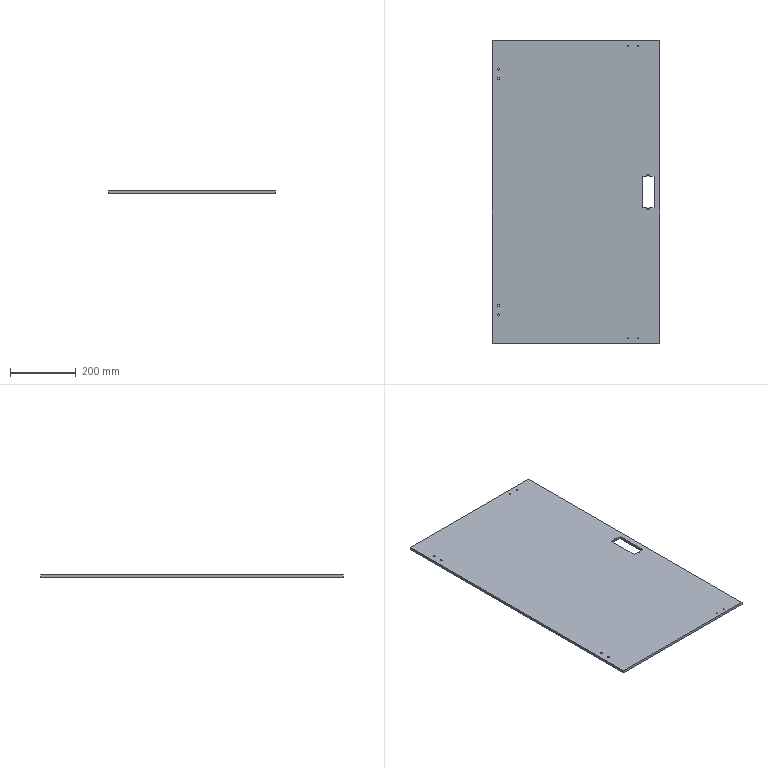Part | STEP file | Left door panel_PN_0007 | 1 solid | 30 faces | box 508.5 x 917 x 8 mm | volume 3700970 mm3 | cylinder 18 | plane 12 | commonest cylinder face diameters 3.3 x8 6.5 x8 8 x2
STEP:
#1=CARTESIAN_POINT('',(-232.,373.5,-4.));
#2=VERTEX_POINT('',#1);
#3=CARTESIAN_POINT('',(-238.5,373.5,-4.));
#4=VERTEX_POINT('',#3);
#5=CARTESIAN_POINT('',(-235.25,373.5,-4.));
#6=DIRECTION('',(0.,0.,-1.));
#7=DIRECTION('',(1.,0.,0.));
#8=AXIS2_PLACEMENT_3D('',#5,#6,#7);
#9=CIRCLE('',#8,3.25);
#10=EDGE_CURVE('',#2,#4,#9,.T.);
#11=ORIENTED_EDGE('',*,*,#10,.T.);
#12=CARTESIAN_POINT('',(-238.5,373.5,4.));
#13=VERTEX_POINT('',#12);
#14=CARTESIAN_POINT('',(-238.5,373.5,-4.));
#15=DIRECTION('',(0.,0.,1.));
#16=VECTOR('',#15,1000.);
#17=LINE('',#14,#16);
#18=EDGE_CURVE('',#4,#13,#17,.T.);
#19=ORIENTED_EDGE('',*,*,#18,.T.);
#20=CARTESIAN_POINT('',(-232.,373.5,4.));
#21=VERTEX_POINT('',#20);
#22=CARTESIAN_POINT('',(-235.25,373.5,4.));
#23=DIRECTION('',(0.,0.,-1.));
#24=DIRECTION('',(1.,0.,0.));
#25=AXIS2_PLACEMENT_3D('',#22,#23,#24);
#26=CIRCLE('',#25,3.25);
#27=EDGE_CURVE('',#21,#13,#26,.T.);
#28=ORIENTED_EDGE('',*,*,#27,.F.);
#29=CARTESIAN_POINT('',(-232.,373.5,-4.));
#30=DIRECTION('',(0.,0.,1.));
#31=VECTOR('',#30,1000.);
#32=LINE('',#29,#31);
#33=EDGE_CURVE('',#2,#21,#32,.T.);
#34=ORIENTED_EDGE('',*,*,#33,.F.);
#35=EDGE_LOOP('',(#11,#19,#28,#34));
#36=FACE_OUTER_BOUND('',#35,.T.);
#37=CARTESIAN_POINT('',(-235.25,373.5,-4.));
#38=DIRECTION('',(0.,0.,1.));
#39=DIRECTION('',(1.,0.,0.));
#40=AXIS2_PLACEMENT_3D('',#37,#38,#39);
#41=CYLINDRICAL_SURFACE('',#40,3.25);
#42=ADVANCED_FACE('',(#36),#41,.F.);
#43=CARTESIAN_POINT('',(-232.,343.5,-4.));
#44=VERTEX_POINT('',#43);
#45=CARTESIAN_POINT('',(-238.5,343.5,-4.));
#46=VERTEX_POINT('',#45);
#47=CARTESIAN_POINT('',(-235.25,343.5,-4.));
#48=DIRECTION('',(0.,0.,-1.));
#49=DIRECTION('',(1.,0.,0.));
#50=AXIS2_PLACEMENT_3D('',#47,#48,#49);
#51=CIRCLE('',#50,3.25);
#52=EDGE_CURVE('',#44,#46,#51,.T.);
#53=ORIENTED_EDGE('',*,*,#52,.T.);
#54=CARTESIAN_POINT('',(-238.5,343.5,4.));
#55=VERTEX_POINT('',#54);
#56=CARTESIAN_POINT('',(-238.5,343.5,-4.));
#57=DIRECTION('',(0.,0.,1.));
#58=VECTOR('',#57,1000.);
#59=LINE('',#56,#58);
#60=EDGE_CURVE('',#46,#55,#59,.T.);
#61=ORIENTED_EDGE('',*,*,#60,.T.);
#62=CARTESIAN_POINT('',(-232.,343.5,4.));
#63=VERTEX_POINT('',#62);
#64=CARTESIAN_POINT('',(-235.25,343.5,4.));
#65=DIRECTION('',(0.,0.,-1.));
#66=DIRECTION('',(1.,0.,0.));
#67=AXIS2_PLACEMENT_3D('',#64,#65,#66);
#68=CIRCLE('',#67,3.25);
#69=EDGE_CURVE('',#63,#55,#68,.T.);
#70=ORIENTED_EDGE('',*,*,#69,.F.);
#71=CARTESIAN_POINT('',(-232.,343.5,-4.));
#72=DIRECTION('',(0.,0.,1.));
#73=VECTOR('',#72,1000.);
#74=LINE('',#71,#73);
#75=EDGE_CURVE('',#44,#63,#74,.T.);
#76=ORIENTED_EDGE('',*,*,#75,.F.);
#77=EDGE_LOOP('',(#53,#61,#70,#76));
#78=FACE_OUTER_BOUND('',#77,.T.);
#79=CARTESIAN_POINT('',(-235.25,343.5,-4.));
#80=DIRECTION('',(0.,0.,1.));
#81=DIRECTION('',(1.,0.,0.));
#82=AXIS2_PLACEMENT_3D('',#79,#80,#81);
#83=CYLINDRICAL_SURFACE('',#82,3.25);
#84=ADVANCED_FACE('',(#78),#83,.F.);
#85=CARTESIAN_POINT('',(-232.,-343.5,-4.));
#86=VERTEX_POINT('',#85);
#87=CARTESIAN_POINT('',(-238.5,-343.5,-4.));
#88=VERTEX_POINT('',#87);
#89=CARTESIAN_POINT('',(-235.25,-343.5,-4.));
#90=DIRECTION('',(0.,0.,-1.));
#91=DIRECTION('',(1.,0.,0.));
#92=AXIS2_PLACEMENT_3D('',#89,#90,#91);
#93=CIRCLE('',#92,3.25);
#94=EDGE_CURVE('',#86,#88,#93,.T.);
#95=ORIENTED_EDGE('',*,*,#94,.T.);
#96=CARTESIAN_POINT('',(-238.5,-343.5,4.));
#97=VERTEX_POINT('',#96);
#98=CARTESIAN_POINT('',(-238.5,-343.5,-4.));
#99=DIRECTION('',(0.,0.,1.));
#100=VECTOR('',#99,1000.);
#101=LINE('',#98,#100);
#102=EDGE_CURVE('',#88,#97,#101,.T.);
#103=ORIENTED_EDGE('',*,*,#102,.T.);
#104=CARTESIAN_POINT('',(-232.,-343.5,4.));
#105=VERTEX_POINT('',#104);
#106=CARTESIAN_POINT('',(-235.25,-343.5,4.));
#107=DIRECTION('',(0.,0.,-1.));
#108=DIRECTION('',(1.,0.,0.));
#109=AXIS2_PLACEMENT_3D('',#106,#107,#108);
#110=CIRCLE('',#109,3.25);
#111=EDGE_CURVE('',#105,#97,#110,.T.);
#112=ORIENTED_EDGE('',*,*,#111,.F.);
#113=CARTESIAN_POINT('',(-232.,-343.5,-4.));
#114=DIRECTION('',(0.,0.,1.));
#115=VECTOR('',#114,1000.);
#116=LINE('',#113,#115);
#117=EDGE_CURVE('',#86,#105,#116,.T.);
#118=ORIENTED_EDGE('',*,*,#117,.F.);
#119=EDGE_LOOP('',(#95,#103,#112,#118));
#120=FACE_OUTER_BOUND('',#119,.T.);
#121=CARTESIAN_POINT('',(-235.25,-343.5,-4.));
#122=DIRECTION('',(0.,0.,1.));
#123=DIRECTION('',(1.,0.,0.));
#124=AXIS2_PLACEMENT_3D('',#121,#122,#123);
#125=CYLINDRICAL_SURFACE('',#124,3.25);
#126=ADVANCED_FACE('',(#120),#125,.F.);
#127=CARTESIAN_POINT('',(-232.,-373.5,-4.));
#128=VERTEX_POINT('',#127);
#129=CARTESIAN_POINT('',(-238.5,-373.5,-4.));
#130=VERTEX_POINT('',#129);
#131=CARTESIAN_POINT('',(-235.25,-373.5,-4.));
#132=DIRECTION('',(0.,0.,-1.));
#133=DIRECTION('',(1.,0.,0.));
#134=AXIS2_PLACEMENT_3D('',#131,#132,#133);
#135=CIRCLE('',#134,3.25);
#136=EDGE_CURVE('',#128,#130,#135,.T.);
#137=ORIENTED_EDGE('',*,*,#136,.T.);
#138=CARTESIAN_POINT('',(-238.5,-373.5,4.));
#139=VERTEX_POINT('',#138);
#140=CARTESIAN_POINT('',(-238.5,-373.5,-4.));
#141=DIRECTION('',(0.,0.,1.));
#142=VECTOR('',#141,1000.);
#143=LINE('',#140,#142);
#144=EDGE_CURVE('',#130,#139,#143,.T.);
#145=ORIENTED_EDGE('',*,*,#144,.T.);
#146=CARTESIAN_POINT('',(-232.,-373.5,4.));
#147=VERTEX_POINT('',#146);
#148=CARTESIAN_POINT('',(-235.25,-373.5,4.));
#149=DIRECTION('',(0.,0.,-1.));
#150=DIRECTION('',(1.,0.,0.));
#151=AXIS2_PLACEMENT_3D('',#148,#149,#150);
#152=CIRCLE('',#151,3.25);
#153=EDGE_CURVE('',#147,#139,#152,.T.);
#154=ORIENTED_EDGE('',*,*,#153,.F.);
#155=CARTESIAN_POINT('',(-232.,-373.5,-4.));
#156=DIRECTION('',(0.,0.,1.));
#157=VECTOR('',#156,1000.);
#158=LINE('',#155,#157);
#159=EDGE_CURVE('',#128,#147,#158,.T.);
#160=ORIENTED_EDGE('',*,*,#159,.F.);
#161=EDGE_LOOP('',(#137,#145,#154,#160));
#162=FACE_OUTER_BOUND('',#161,.T.);
#163=CARTESIAN_POINT('',(-235.25,-373.5,-4.));
#164=DIRECTION('',(0.,0.,1.));
#165=DIRECTION('',(1.,0.,0.));
#166=AXIS2_PLACEMENT_3D('',#163,#164,#165);
#167=CYLINDRICAL_SURFACE('',#166,3.25);
#168=ADVANCED_FACE('',(#162),#167,.F.);
#169=CARTESIAN_POINT('',(160.9,-444.5,4.));
#170=VERTEX_POINT('',#169);
#171=CARTESIAN_POINT('',(157.6,-444.5,4.));
#172=VERTEX_POINT('',#171);
#173=CARTESIAN_POINT('',(159.25,-444.5,4.));
#174=DIRECTION('',(0.,0.,-1.));
#175=DIRECTION('',(-1.,0.,0.));
#176=AXIS2_PLACEMENT_3D('',#173,#174,#175);
#177=CIRCLE('',#176,1.65);
#178=EDGE_CURVE('',#170,#172,#177,.T.);
#179=ORIENTED_EDGE('',*,*,#178,.F.);
#180=CARTESIAN_POINT('',(160.9,-444.5,-4.));
#181=VERTEX_POINT('',#180);
#182=CARTESIAN_POINT('',(160.9,-444.5,-4.));
#183=DIRECTION('',(0.,0.,-1.));
#184=VECTOR('',#183,1000.);
#185=LINE('',#182,#184);
#186=EDGE_CURVE('',#170,#181,#185,.T.);
#187=ORIENTED_EDGE('',*,*,#186,.T.);
#188=CARTESIAN_POINT('',(157.6,-444.5,-4.));
#189=VERTEX_POINT('',#188);
#190=CARTESIAN_POINT('',(159.25,-444.5,-4.));
#191=DIRECTION('',(0.,0.,-1.));
#192=DIRECTION('',(-1.,0.,0.));
#193=AXIS2_PLACEMENT_3D('',#190,#191,#192);
#194=CIRCLE('',#193,1.65);
#195=EDGE_CURVE('',#181,#189,#194,.T.);
#196=ORIENTED_EDGE('',*,*,#195,.T.);
#197=CARTESIAN_POINT('',(157.6,-444.5,-4.));
#198=DIRECTION('',(0.,0.,-1.));
#199=VECTOR('',#198,1000.);
#200=LINE('',#197,#199);
#201=EDGE_CURVE('',#172,#189,#200,.T.);
#202=ORIENTED_EDGE('',*,*,#201,.F.);
#203=EDGE_LOOP('',(#179,#187,#196,#202));
#204=FACE_OUTER_BOUND('',#203,.T.);
#205=CARTESIAN_POINT('',(159.25,-444.5,-4.));
#206=DIRECTION('',(0.,0.,-1.));
#207=DIRECTION('',(-1.,0.,0.));
#208=AXIS2_PLACEMENT_3D('',#205,#206,#207);
#209=CYLINDRICAL_SURFACE('',#208,1.65);
#210=ADVANCED_FACE('',(#204),#209,.F.);
#211=CARTESIAN_POINT('',(190.9,-444.5,4.));
#212=VERTEX_POINT('',#211);
#213=CARTESIAN_POINT('',(187.6,-444.5,4.));
#214=VERTEX_POINT('',#213);
#215=CARTESIAN_POINT('',(189.25,-444.5,4.));
#216=DIRECTION('',(0.,0.,-1.));
#217=DIRECTION('',(-1.,0.,0.));
#218=AXIS2_PLACEMENT_3D('',#215,#216,#217);
#219=CIRCLE('',#218,1.65);
#220=EDGE_CURVE('',#212,#214,#219,.T.);
#221=ORIENTED_EDGE('',*,*,#220,.F.);
#222=CARTESIAN_POINT('',(190.9,-444.5,-4.));
#223=VERTEX_POINT('',#222);
#224=CARTESIAN_POINT('',(190.9,-444.5,-4.));
#225=DIRECTION('',(0.,0.,-1.));
#226=VECTOR('',#225,1000.);
#227=LINE('',#224,#226);
#228=EDGE_CURVE('',#212,#223,#227,.T.);
#229=ORIENTED_EDGE('',*,*,#228,.T.);
#230=CARTESIAN_POINT('',(187.6,-444.5,-4.));
#231=VERTEX_POINT('',#230);
#232=CARTESIAN_POINT('',(189.25,-444.5,-4.));
#233=DIRECTION('',(0.,0.,-1.));
#234=DIRECTION('',(-1.,0.,0.));
#235=AXIS2_PLACEMENT_3D('',#232,#233,#234);
#236=CIRCLE('',#235,1.65);
#237=EDGE_CURVE('',#223,#231,#236,.T.);
#238=ORIENTED_EDGE('',*,*,#237,.T.);
#239=CARTESIAN_POINT('',(187.6,-444.5,-4.));
#240=DIRECTION('',(0.,0.,-1.));
#241=VECTOR('',#240,1000.);
#242=LINE('',#239,#241);
#243=EDGE_CURVE('',#214,#231,#242,.T.);
#244=ORIENTED_EDGE('',*,*,#243,.F.);
#245=EDGE_LOOP('',(#221,#229,#238,#244));
#246=FACE_OUTER_BOUND('',#245,.T.);
#247=CARTESIAN_POINT('',(189.25,-444.5,-4.));
#248=DIRECTION('',(0.,0.,-1.));
#249=DIRECTION('',(-1.,0.,0.));
#250=AXIS2_PLACEMENT_3D('',#247,#248,#249);
#251=CYLINDRICAL_SURFACE('',#250,1.65);
#252=ADVANCED_FACE('',(#246),#251,.F.);
#253=CARTESIAN_POINT('',(160.9,443.5,4.));
#254=VERTEX_POINT('',#253);
#255=CARTESIAN_POINT('',(157.6,443.5,4.));
#256=VERTEX_POINT('',#255);
#257=CARTESIAN_POINT('',(159.25,443.5,4.));
#258=DIRECTION('',(0.,0.,-1.));
#259=DIRECTION('',(-1.,0.,0.));
#260=AXIS2_PLACEMENT_3D('',#257,#258,#259);
#261=CIRCLE('',#260,1.65);
#262=EDGE_CURVE('',#254,#256,#261,.T.);
#263=ORIENTED_EDGE('',*,*,#262,.F.);
#264=CARTESIAN_POINT('',(160.9,443.5,-4.));
#265=VERTEX_POINT('',#264);
#266=CARTESIAN_POINT('',(160.9,443.5,-4.));
#267=DIRECTION('',(0.,0.,-1.));
#268=VECTOR('',#267,1000.);
#269=LINE('',#266,#268);
#270=EDGE_CURVE('',#254,#265,#269,.T.);
#271=ORIENTED_EDGE('',*,*,#270,.T.);
#272=CARTESIAN_POINT('',(157.6,443.5,-4.));
#273=VERTEX_POINT('',#272);
#274=CARTESIAN_POINT('',(159.25,443.5,-4.));
#275=DIRECTION('',(0.,0.,-1.));
#276=DIRECTION('',(-1.,0.,0.));
#277=AXIS2_PLACEMENT_3D('',#274,#275,#276);
#278=CIRCLE('',#277,1.65);
#279=EDGE_CURVE('',#265,#273,#278,.T.);
#280=ORIENTED_EDGE('',*,*,#279,.T.);
#281=CARTESIAN_POINT('',(157.6,443.5,-4.));
#282=DIRECTION('',(0.,0.,-1.));
#283=VECTOR('',#282,1000.);
#284=LINE('',#281,#283);
#285=EDGE_CURVE('',#256,#273,#284,.T.);
#286=ORIENTED_EDGE('',*,*,#285,.F.);
#287=EDGE_LOOP('',(#263,#271,#280,#286));
#288=FACE_OUTER_BOUND('',#287,.T.);
#289=CARTESIAN_POINT('',(159.25,443.5,-4.));
#290=DIRECTION('',(0.,0.,-1.));
#291=DIRECTION('',(-1.,0.,0.));
#292=AXIS2_PLACEMENT_3D('',#289,#290,#291);
#293=CYLINDRICAL_SURFACE('',#292,1.65);
#294=ADVANCED_FACE('',(#288),#293,.F.);
#295=CARTESIAN_POINT('',(190.9,443.5,4.));
#296=VERTEX_POINT('',#295);
#297=CARTESIAN_POINT('',(187.6,443.5,4.));
#298=VERTEX_POINT('',#297);
#299=CARTESIAN_POINT('',(189.25,443.5,4.));
#300=DIRECTION('',(0.,0.,-1.));
#301=DIRECTION('',(-1.,0.,0.));
#302=AXIS2_PLACEMENT_3D('',#299,#300,#301);
#303=CIRCLE('',#302,1.65);
#304=EDGE_CURVE('',#296,#298,#303,.T.);
#305=ORIENTED_EDGE('',*,*,#304,.F.);
#306=CARTESIAN_POINT('',(190.9,443.5,-4.));
#307=VERTEX_POINT('',#306);
#308=CARTESIAN_POINT('',(190.9,443.5,-4.));
#309=DIRECTION('',(0.,0.,-1.));
#310=VECTOR('',#309,1000.);
#311=LINE('',#308,#310);
#312=EDGE_CURVE('',#296,#307,#311,.T.);
#313=ORIENTED_EDGE('',*,*,#312,.T.);
#314=CARTESIAN_POINT('',(187.6,443.5,-4.));
#315=VERTEX_POINT('',#314);
#316=CARTESIAN_POINT('',(189.25,443.5,-4.));
#317=DIRECTION('',(0.,0.,-1.));
#318=DIRECTION('',(-1.,0.,0.));
#319=AXIS2_PLACEMENT_3D('',#316,#317,#318);
#320=CIRCLE('',#319,1.65);
#321=EDGE_CURVE('',#307,#315,#320,.T.);
#322=ORIENTED_EDGE('',*,*,#321,.T.);
#323=CARTESIAN_POINT('',(187.6,443.5,-4.));
#324=DIRECTION('',(0.,0.,-1.));
#325=VECTOR('',#324,1000.);
#326=LINE('',#323,#325);
#327=EDGE_CURVE('',#298,#315,#326,.T.);
#328=ORIENTED_EDGE('',*,*,#327,.F.);
#329=EDGE_LOOP('',(#305,#313,#322,#328));
#330=FACE_OUTER_BOUND('',#329,.T.);
#331=CARTESIAN_POINT('',(189.25,443.5,-4.));
#332=DIRECTION('',(0.,0.,-1.));
#333=DIRECTION('',(-1.,0.,0.));
#334=AXIS2_PLACEMENT_3D('',#331,#332,#333);
#335=CYLINDRICAL_SURFACE('',#334,1.65);
#336=ADVANCED_FACE('',(#330),#335,.F.);
#337=CARTESIAN_POINT('',(215.25,48.,-4.));
#338=VERTEX_POINT('',#337);
#339=CARTESIAN_POINT('',(223.25,48.,-4.));
#340=VERTEX_POINT('',#339);
#341=CARTESIAN_POINT('',(219.25,48.,-4.));
#342=DIRECTION('',(0.,0.,-1.));
#343=DIRECTION('',(1.,0.,0.));
#344=AXIS2_PLACEMENT_3D('',#341,#342,#343);
#345=CIRCLE('',#344,4.);
#346=EDGE_CURVE('',#338,#340,#345,.T.);
#347=ORIENTED_EDGE('',*,*,#346,.F.);
#348=CARTESIAN_POINT('',(201.25,48.,-4.));
#349=VERTEX_POINT('',#348);
#350=CARTESIAN_POINT('',(0.,48.,-4.));
#351=DIRECTION('',(1.,0.,0.));
#352=VECTOR('',#351,1000.);
#353=LINE('',#350,#352);
#354=EDGE_CURVE('',#349,#338,#353,.T.);
#355=ORIENTED_EDGE('',*,*,#354,.F.);
#356=CARTESIAN_POINT('',(201.25,-48.,-4.));
#357=VERTEX_POINT('',#356);
#358=CARTESIAN_POINT('',(201.25,0.,-4.));
#359=DIRECTION('',(0.,1.,0.));
#360=VECTOR('',#359,1000.);
#361=LINE('',#358,#360);
#362=EDGE_CURVE('',#357,#349,#361,.T.);
#363=ORIENTED_EDGE('',*,*,#362,.F.);
#364=CARTESIAN_POINT('',(215.25,-48.,-4.));
#365=VERTEX_POINT('',#364);
#366=CARTESIAN_POINT('',(0.,-48.,-4.));
#367=DIRECTION('',(-1.,0.,0.));
#368=VECTOR('',#367,1000.);
#369=LINE('',#366,#368);
#370=EDGE_CURVE('',#365,#357,#369,.T.);
#371=ORIENTED_EDGE('',*,*,#370,.F.);
#372=CARTESIAN_POINT('',(223.25,-48.,-4.));
#373=VERTEX_POINT('',#372);
#374=CARTESIAN_POINT('',(219.25,-48.,-4.));
#375=DIRECTION('',(0.,0.,-1.));
#376=DIRECTION('',(1.,0.,0.));
#377=AXIS2_PLACEMENT_3D('',#374,#375,#376);
#378=CIRCLE('',#377,4.);
#379=EDGE_CURVE('',#373,#365,#378,.T.);
#380=ORIENTED_EDGE('',*,*,#379,.F.);
#381=CARTESIAN_POINT('',(237.25,-48.,-4.));
#382=VERTEX_POINT('',#381);
#383=CARTESIAN_POINT('',(0.,-48.,-4.));
#384=DIRECTION('',(-1.,0.,0.));
#385=VECTOR('',#384,1000.);
#386=LINE('',#383,#385);
#387=EDGE_CURVE('',#382,#373,#386,.T.);
#388=ORIENTED_EDGE('',*,*,#387,.F.);
#389=CARTESIAN_POINT('',(237.25,48.,-4.));
#390=VERTEX_POINT('',#389);
#391=CARTESIAN_POINT('',(237.25,0.,-4.));
#392=DIRECTION('',(0.,-1.,0.));
#393=VECTOR('',#392,1000.);
#394=LINE('',#391,#393);
#395=EDGE_CURVE('',#390,#382,#394,.T.);
#396=ORIENTED_EDGE('',*,*,#395,.F.);
#397=CARTESIAN_POINT('',(0.,48.,-4.));
#398=DIRECTION('',(1.,0.,0.));
#399=VECTOR('',#398,1000.);
#400=LINE('',#397,#399);
#401=EDGE_CURVE('',#340,#390,#400,.T.);
#402=ORIENTED_EDGE('',*,*,#401,.F.);
#403=EDGE_LOOP('',(#347,#355,#363,#371,#380,#388,#396,#402));
#404=FACE_BOUND('',#403,.T.);
#405=CARTESIAN_POINT('',(-254.25,-458.5,-4.));
#406=VERTEX_POINT('',#405);
#407=CARTESIAN_POINT('',(254.25,-458.5,-4.));
#408=VERTEX_POINT('',#407);
#409=CARTESIAN_POINT('',(0.,-458.5,-4.));
#410=DIRECTION('',(1.,0.,0.));
#411=VECTOR('',#410,1000.);
#412=LINE('',#409,#411);
#413=EDGE_CURVE('',#406,#408,#412,.T.);
#414=ORIENTED_EDGE('',*,*,#413,.F.);
#415=CARTESIAN_POINT('',(-254.25,458.5,-4.));
#416=VERTEX_POINT('',#415);
#417=CARTESIAN_POINT('',(-254.25,0.,-4.));
#418=DIRECTION('',(0.,-1.,0.));
#419=VECTOR('',#418,1000.);
#420=LINE('',#417,#419);
#421=EDGE_CURVE('',#416,#406,#420,.T.);
#422=ORIENTED_EDGE('',*,*,#421,.F.);
#423=CARTESIAN_POINT('',(254.25,458.5,-4.));
#424=VERTEX_POINT('',#423);
#425=CARTESIAN_POINT('',(0.,458.5,-4.));
#426=DIRECTION('',(-1.,0.,0.));
#427=VECTOR('',#426,1000.);
#428=LINE('',#425,#427);
#429=EDGE_CURVE('',#424,#416,#428,.T.);
#430=ORIENTED_EDGE('',*,*,#429,.F.);
#431=CARTESIAN_POINT('',(254.25,0.,-4.));
#432=DIRECTION('',(0.,1.,0.));
#433=VECTOR('',#432,1000.);
#434=LINE('',#431,#433);
#435=EDGE_CURVE('',#408,#424,#434,.T.);
#436=ORIENTED_EDGE('',*,*,#435,.F.);
#437=EDGE_LOOP('',(#414,#422,#430,#436));
#438=FACE_OUTER_BOUND('',#437,.T.);
#439=ORIENTED_EDGE('',*,*,#10,.F.);
#440=CARTESIAN_POINT('',(-235.25,373.5,-4.));
#441=DIRECTION('',(0.,0.,-1.));
#442=DIRECTION('',(1.,0.,0.));
#443=AXIS2_PLACEMENT_3D('',#440,#441,#442);
#444=CIRCLE('',#443,3.25);
#445=EDGE_CURVE('',#4,#2,#444,.T.);
#446=ORIENTED_EDGE('',*,*,#445,.F.);
#447=EDGE_LOOP('',(#439,#446));
#448=FACE_BOUND('',#447,.T.);
#449=ORIENTED_EDGE('',*,*,#52,.F.);
#450=CARTESIAN_POINT('',(-235.25,343.5,-4.));
#451=DIRECTION('',(0.,0.,-1.));
#452=DIRECTION('',(1.,0.,0.));
#453=AXIS2_PLACEMENT_3D('',#450,#451,#452);
#454=CIRCLE('',#453,3.25);
#455=EDGE_CURVE('',#46,#44,#454,.T.);
#456=ORIENTED_EDGE('',*,*,#455,.F.);
#457=EDGE_LOOP('',(#449,#456));
#458=FACE_BOUND('',#457,.T.);
#459=ORIENTED_EDGE('',*,*,#94,.F.);
#460=CARTESIAN_POINT('',(-235.25,-343.5,-4.));
#461=DIRECTION('',(0.,0.,-1.));
#462=DIRECTION('',(1.,0.,0.));
#463=AXIS2_PLACEMENT_3D('',#460,#461,#462);
#464=CIRCLE('',#463,3.25);
#465=EDGE_CURVE('',#88,#86,#464,.T.);
#466=ORIENTED_EDGE('',*,*,#465,.F.);
#467=EDGE_LOOP('',(#459,#466));
#468=FACE_BOUND('',#467,.T.);
#469=ORIENTED_EDGE('',*,*,#136,.F.);
#470=CARTESIAN_POINT('',(-235.25,-373.5,-4.));
#471=DIRECTION('',(0.,0.,-1.));
#472=DIRECTION('',(1.,0.,0.));
#473=AXIS2_PLACEMENT_3D('',#470,#471,#472);
#474=CIRCLE('',#473,3.25);
#475=EDGE_CURVE('',#130,#128,#474,.T.);
#476=ORIENTED_EDGE('',*,*,#475,.F.);
#477=EDGE_LOOP('',(#469,#476));
#478=FACE_BOUND('',#477,.T.);
#479=CARTESIAN_POINT('',(159.25,-444.5,-4.));
#480=DIRECTION('',(0.,0.,-1.));
#481=DIRECTION('',(-1.,0.,0.));
#482=AXIS2_PLACEMENT_3D('',#479,#480,#481);
#483=CIRCLE('',#482,1.65);
#484=EDGE_CURVE('',#189,#181,#483,.T.);
#485=ORIENTED_EDGE('',*,*,#484,.F.);
#486=ORIENTED_EDGE('',*,*,#195,.F.);
#487=EDGE_LOOP('',(#485,#486));
#488=FACE_BOUND('',#487,.T.);
#489=CARTESIAN_POINT('',(189.25,-444.5,-4.));
#490=DIRECTION('',(0.,0.,-1.));
#491=DIRECTION('',(-1.,0.,0.));
#492=AXIS2_PLACEMENT_3D('',#489,#490,#491);
#493=CIRCLE('',#492,1.65);
#494=EDGE_CURVE('',#231,#223,#493,.T.);
#495=ORIENTED_EDGE('',*,*,#494,.F.);
#496=ORIENTED_EDGE('',*,*,#237,.F.);
#497=EDGE_LOOP('',(#495,#496));
#498=FACE_BOUND('',#497,.T.);
#499=CARTESIAN_POINT('',(159.25,443.5,-4.));
#500=DIRECTION('',(0.,0.,-1.));
#501=DIRECTION('',(-1.,0.,0.));
#502=AXIS2_PLACEMENT_3D('',#499,#500,#501);
#503=CIRCLE('',#502,1.65);
#504=EDGE_CURVE('',#273,#265,#503,.T.);
#505=ORIENTED_EDGE('',*,*,#504,.F.);
#506=ORIENTED_EDGE('',*,*,#279,.F.);
#507=EDGE_LOOP('',(#505,#506));
#508=FACE_BOUND('',#507,.T.);
#509=CARTESIAN_POINT('',(189.25,443.5,-4.));
#510=DIRECTION('',(0.,0.,-1.));
#511=DIRECTION('',(-1.,0.,0.));
#512=AXIS2_PLACEMENT_3D('',#509,#510,#511);
#513=CIRCLE('',#512,1.65);
#514=EDGE_CURVE('',#315,#307,#513,.T.);
#515=ORIENTED_EDGE('',*,*,#514,.F.);
#516=ORIENTED_EDGE('',*,*,#321,.F.);
#517=EDGE_LOOP('',(#515,#516));
#518=FACE_BOUND('',#517,.T.);
#519=CARTESIAN_POINT('',(0.,0.,-4.));
#520=DIRECTION('',(0.,0.,1.));
#521=DIRECTION('',(1.,0.,0.));
#522=AXIS2_PLACEMENT_3D('',#519,#520,#521);
#523=PLANE('',#522);
#524=ADVANCED_FACE('',(#404,#438,#448,#458,#468,#478,#488,#498,#508,#518),#523,.F.);
#525=ORIENTED_EDGE('',*,*,#401,.T.);
#526=CARTESIAN_POINT('',(237.25,48.,4.));
#527=VERTEX_POINT('',#526);
#528=CARTESIAN_POINT('',(237.25,48.,-4.));
#529=DIRECTION('',(0.,0.,1.));
#530=VECTOR('',#529,1000.);
#531=LINE('',#528,#530);
#532=EDGE_CURVE('',#390,#527,#531,.T.);
#533=ORIENTED_EDGE('',*,*,#532,.T.);
#534=CARTESIAN_POINT('',(223.25,48.,4.));
#535=VERTEX_POINT('',#534);
#536=CARTESIAN_POINT('',(0.,48.,4.));
#537=DIRECTION('',(-1.,0.,0.));
#538=VECTOR('',#537,1000.);
#539=LINE('',#536,#538);
#540=EDGE_CURVE('',#527,#535,#539,.T.);
#541=ORIENTED_EDGE('',*,*,#540,.T.);
#542=CARTESIAN_POINT('',(223.25,48.,-4.));
#543=DIRECTION('',(0.,0.,-1.));
#544=VECTOR('',#543,1000.);
#545=LINE('',#542,#544);
#546=EDGE_CURVE('',#535,#340,#545,.T.);
#547=ORIENTED_EDGE('',*,*,#546,.T.);
#548=EDGE_LOOP('',(#525,#533,#541,#547));
#549=FACE_OUTER_BOUND('',#548,.T.);
#550=CARTESIAN_POINT('',(0.,48.,-4.));
#551=DIRECTION('',(0.,-1.,0.));
#552=DIRECTION('',(1.,0.,0.));
#553=AXIS2_PLACEMENT_3D('',#550,#551,#552);
#554=PLANE('',#553);
#555=ADVANCED_FACE('',(#549),#554,.T.);
#556=CARTESIAN_POINT('',(215.25,48.,4.));
#557=VERTEX_POINT('',#556);
#558=CARTESIAN_POINT('',(215.25,48.,-4.));
#559=DIRECTION('',(0.,0.,1.));
#560=VECTOR('',#559,1000.);
#561=LINE('',#558,#560);
#562=EDGE_CURVE('',#338,#557,#561,.T.);
#563=ORIENTED_EDGE('',*,*,#562,.F.);
#564=ORIENTED_EDGE('',*,*,#346,.T.);
#565=ORIENTED_EDGE('',*,*,#546,.F.);
#566=CARTESIAN_POINT('',(219.25,48.,4.));
#567=DIRECTION('',(0.,0.,-1.));
#568=DIRECTION('',(1.,0.,0.));
#569=AXIS2_PLACEMENT_3D('',#566,#567,#568);
#570=CIRCLE('',#569,4.);
#571=EDGE_CURVE('',#557,#535,#570,.T.);
#572=ORIENTED_EDGE('',*,*,#571,.F.);
#573=EDGE_LOOP('',(#563,#564,#565,#572));
#574=FACE_OUTER_BOUND('',#573,.T.);
#575=CARTESIAN_POINT('',(219.25,48.,-4.));
#576=DIRECTION('',(0.,0.,1.));
#577=DIRECTION('',(1.,0.,0.));
#578=AXIS2_PLACEMENT_3D('',#575,#576,#577);
#579=CYLINDRICAL_SURFACE('',#578,4.);
#580=ADVANCED_FACE('',(#574),#579,.F.);
#581=ORIENTED_EDGE('',*,*,#354,.T.);
#582=ORIENTED_EDGE('',*,*,#562,.T.);
#583=CARTESIAN_POINT('',(201.25,48.,4.));
#584=VERTEX_POINT('',#583);
#585=CARTESIAN_POINT('',(0.,48.,4.));
#586=DIRECTION('',(-1.,0.,0.));
#587=VECTOR('',#586,1000.);
#588=LINE('',#585,#587);
#589=EDGE_CURVE('',#557,#584,#588,.T.);
#590=ORIENTED_EDGE('',*,*,#589,.T.);
#591=CARTESIAN_POINT('',(201.25,48.,-4.));
#592=DIRECTION('',(0.,0.,-1.));
#593=VECTOR('',#592,1000.);
#594=LINE('',#591,#593);
#595=EDGE_CURVE('',#584,#349,#594,.T.);
#596=ORIENTED_EDGE('',*,*,#595,.T.);
#597=EDGE_LOOP('',(#581,#582,#590,#596));
#598=FACE_OUTER_BOUND('',#597,.T.);
#599=CARTESIAN_POINT('',(0.,48.,-4.));
#600=DIRECTION('',(0.,-1.,0.));
#601=DIRECTION('',(0.,0.,-1.));
#602=AXIS2_PLACEMENT_3D('',#599,#600,#601);
#603=PLANE('',#602);
#604=ADVANCED_FACE('',(#598),#603,.T.);
#605=CARTESIAN_POINT('',(201.25,-48.,4.));
#606=VERTEX_POINT('',#605);
#607=CARTESIAN_POINT('',(201.25,-48.,-4.));
#608=DIRECTION('',(0.,0.,1.));
#609=VECTOR('',#608,1000.);
#610=LINE('',#607,#609);
#611=EDGE_CURVE('',#357,#606,#610,.T.);
#612=ORIENTED_EDGE('',*,*,#611,.F.);
#613=ORIENTED_EDGE('',*,*,#362,.T.);
#614=ORIENTED_EDGE('',*,*,#595,.F.);
#615=CARTESIAN_POINT('',(201.25,0.,4.));
#616=DIRECTION('',(0.,1.,0.));
#617=VECTOR('',#616,1000.);
#618=LINE('',#615,#617);
#619=EDGE_CURVE('',#606,#584,#618,.T.);
#620=ORIENTED_EDGE('',*,*,#619,.F.);
#621=EDGE_LOOP('',(#612,#613,#614,#620));
#622=FACE_OUTER_BOUND('',#621,.T.);
#623=CARTESIAN_POINT('',(201.25,0.,-4.));
#624=DIRECTION('',(-1.,0.,0.));
#625=DIRECTION('',(0.,-1.,0.));
#626=AXIS2_PLACEMENT_3D('',#623,#624,#625);
#627=PLANE('',#626);
#628=ADVANCED_FACE('',(#622),#627,.F.);
#629=CARTESIAN_POINT('',(215.25,-48.,4.));
#630=VERTEX_POINT('',#629);
#631=CARTESIAN_POINT('',(215.25,-48.,-4.));
#632=DIRECTION('',(0.,0.,1.));
#633=VECTOR('',#632,1000.);
#634=LINE('',#631,#633);
#635=EDGE_CURVE('',#365,#630,#634,.T.);
#636=ORIENTED_EDGE('',*,*,#635,.F.);
#637=ORIENTED_EDGE('',*,*,#370,.T.);
#638=ORIENTED_EDGE('',*,*,#611,.T.);
#639=CARTESIAN_POINT('',(0.,-48.,4.));
#640=DIRECTION('',(-1.,0.,0.));
#641=VECTOR('',#640,1000.);
#642=LINE('',#639,#641);
#643=EDGE_CURVE('',#630,#606,#642,.T.);
#644=ORIENTED_EDGE('',*,*,#643,.F.);
#645=EDGE_LOOP('',(#636,#637,#638,#644));
#646=FACE_OUTER_BOUND('',#645,.T.);
#647=CARTESIAN_POINT('',(0.,-48.,-4.));
#648=DIRECTION('',(0.,-1.,0.));
#649=DIRECTION('',(0.,0.,-1.));
#650=AXIS2_PLACEMENT_3D('',#647,#648,#649);
#651=PLANE('',#650);
#652=ADVANCED_FACE('',(#646),#651,.F.);
#653=CARTESIAN_POINT('',(223.25,-48.,4.));
#654=VERTEX_POINT('',#653);
#655=CARTESIAN_POINT('',(223.25,-48.,-4.));
#656=DIRECTION('',(0.,0.,1.));
#657=VECTOR('',#656,1000.);
#658=LINE('',#655,#657);
#659=EDGE_CURVE('',#373,#654,#658,.T.);
#660=ORIENTED_EDGE('',*,*,#659,.F.);
#661=ORIENTED_EDGE('',*,*,#379,.T.);
#662=ORIENTED_EDGE('',*,*,#635,.T.);
#663=CARTESIAN_POINT('',(219.25,-48.,4.));
#664=DIRECTION('',(0.,0.,-1.));
#665=DIRECTION('',(1.,0.,0.));
#666=AXIS2_PLACEMENT_3D('',#663,#664,#665);
#667=CIRCLE('',#666,4.);
#668=EDGE_CURVE('',#654,#630,#667,.T.);
#669=ORIENTED_EDGE('',*,*,#668,.F.);
#670=EDGE_LOOP('',(#660,#661,#662,#669));
#671=FACE_OUTER_BOUND('',#670,.T.);
#672=CARTESIAN_POINT('',(219.25,-48.,-4.));
#673=DIRECTION('',(0.,0.,1.));
#674=DIRECTION('',(1.,0.,0.));
#675=AXIS2_PLACEMENT_3D('',#672,#673,#674);
#676=CYLINDRICAL_SURFACE('',#675,4.);
#677=ADVANCED_FACE('',(#671),#676,.F.);
#678=CARTESIAN_POINT('',(237.25,-48.,4.));
#679=VERTEX_POINT('',#678);
#680=CARTESIAN_POINT('',(237.25,-48.,-4.));
#681=DIRECTION('',(0.,0.,1.));
#682=VECTOR('',#681,1000.);
#683=LINE('',#680,#682);
#684=EDGE_CURVE('',#382,#679,#683,.T.);
#685=ORIENTED_EDGE('',*,*,#684,.F.);
#686=ORIENTED_EDGE('',*,*,#387,.T.);
#687=ORIENTED_EDGE('',*,*,#659,.T.);
#688=CARTESIAN_POINT('',(0.,-48.,4.));
#689=DIRECTION('',(-1.,0.,0.));
#690=VECTOR('',#689,1000.);
#691=LINE('',#688,#690);
#692=EDGE_CURVE('',#679,#654,#691,.T.);
#693=ORIENTED_EDGE('',*,*,#692,.F.);
#694=EDGE_LOOP('',(#685,#686,#687,#693));
#695=FACE_OUTER_BOUND('',#694,.T.);
#696=CARTESIAN_POINT('',(0.,-48.,-4.));
#697=DIRECTION('',(0.,-1.,0.));
#698=DIRECTION('',(0.,0.,-1.));
#699=AXIS2_PLACEMENT_3D('',#696,#697,#698);
#700=PLANE('',#699);
#701=ADVANCED_FACE('',(#695),#700,.F.);
#702=ORIENTED_EDGE('',*,*,#395,.T.);
#703=ORIENTED_EDGE('',*,*,#684,.T.);
#704=CARTESIAN_POINT('',(237.25,0.,4.));
#705=DIRECTION('',(0.,1.,0.));
#706=VECTOR('',#705,1000.);
#707=LINE('',#704,#706);
#708=EDGE_CURVE('',#679,#527,#707,.T.);
#709=ORIENTED_EDGE('',*,*,#708,.T.);
#710=ORIENTED_EDGE('',*,*,#532,.F.);
#711=EDGE_LOOP('',(#702,#703,#709,#710));
#712=FACE_OUTER_BOUND('',#711,.T.);
#713=CARTESIAN_POINT('',(237.25,0.,-4.));
#714=DIRECTION('',(-1.,0.,0.));
#715=DIRECTION('',(0.,-1.,0.));
#716=AXIS2_PLACEMENT_3D('',#713,#714,#715);
#717=PLANE('',#716);
#718=ADVANCED_FACE('',(#712),#717,.T.);
#719=CARTESIAN_POINT('',(254.25,458.5,4.));
#720=VERTEX_POINT('',#719);
#721=CARTESIAN_POINT('',(254.25,458.5,4.));
#722=DIRECTION('',(0.,0.,-1.));
#723=VECTOR('',#722,1000.);
#724=LINE('',#721,#723);
#725=EDGE_CURVE('',#720,#424,#724,.T.);
#726=ORIENTED_EDGE('',*,*,#725,.F.);
#727=CARTESIAN_POINT('',(254.25,-458.5,4.));
#728=VERTEX_POINT('',#727);
#729=CARTESIAN_POINT('',(254.25,458.5,4.));
#730=DIRECTION('',(0.,1.,0.));
#731=VECTOR('',#730,1000.);
#732=LINE('',#729,#731);
#733=EDGE_CURVE('',#728,#720,#732,.T.);
#734=ORIENTED_EDGE('',*,*,#733,.F.);
#735=CARTESIAN_POINT('',(254.25,-458.5,4.));
#736=DIRECTION('',(0.,0.,1.));
#737=VECTOR('',#736,1000.);
#738=LINE('',#735,#737);
#739=EDGE_CURVE('',#408,#728,#738,.T.);
#740=ORIENTED_EDGE('',*,*,#739,.F.);
#741=ORIENTED_EDGE('',*,*,#435,.T.);
#742=EDGE_LOOP('',(#726,#734,#740,#741));
#743=FACE_OUTER_BOUND('',#742,.T.);
#744=CARTESIAN_POINT('',(254.25,458.5,4.));
#745=DIRECTION('',(-1.,0.,0.));
#746=DIRECTION('',(0.,-1.,0.));
#747=AXIS2_PLACEMENT_3D('',#744,#745,#746);
#748=PLANE('',#747);
#749=ADVANCED_FACE('',(#743),#748,.F.);
#750=ORIENTED_EDGE('',*,*,#739,.T.);
#751=CARTESIAN_POINT('',(-254.25,-458.5,4.));
#752=VERTEX_POINT('',#751);
#753=CARTESIAN_POINT('',(-254.25,-458.5,4.));
#754=DIRECTION('',(1.,0.,0.));
#755=VECTOR('',#754,1000.);
#756=LINE('',#753,#755);
#757=EDGE_CURVE('',#752,#728,#756,.T.);
#758=ORIENTED_EDGE('',*,*,#757,.F.);
#759=CARTESIAN_POINT('',(-254.25,-458.5,4.));
#760=DIRECTION('',(0.,0.,1.));
#761=VECTOR('',#760,1000.);
#762=LINE('',#759,#761);
#763=EDGE_CURVE('',#406,#752,#762,.T.);
#764=ORIENTED_EDGE('',*,*,#763,.F.);
#765=ORIENTED_EDGE('',*,*,#413,.T.);
#766=EDGE_LOOP('',(#750,#758,#764,#765));
#767=FACE_OUTER_BOUND('',#766,.T.);
#768=CARTESIAN_POINT('',(-254.25,-458.5,4.));
#769=DIRECTION('',(0.,1.,0.));
#770=DIRECTION('',(0.,0.,1.));
#771=AXIS2_PLACEMENT_3D('',#768,#769,#770);
#772=PLANE('',#771);
#773=ADVANCED_FACE('',(#767),#772,.F.);
#774=ORIENTED_EDGE('',*,*,#763,.T.);
#775=CARTESIAN_POINT('',(-254.25,458.5,4.));
#776=VERTEX_POINT('',#775);
#777=CARTESIAN_POINT('',(-254.25,458.5,4.));
#778=DIRECTION('',(0.,-1.,0.));
#779=VECTOR('',#778,1000.);
#780=LINE('',#777,#779);
#781=EDGE_CURVE('',#776,#752,#780,.T.);
#782=ORIENTED_EDGE('',*,*,#781,.F.);
#783=CARTESIAN_POINT('',(-254.25,458.5,4.));
#784=DIRECTION('',(0.,0.,1.));
#785=VECTOR('',#784,1000.);
#786=LINE('',#783,#785);
#787=EDGE_CURVE('',#416,#776,#786,.T.);
#788=ORIENTED_EDGE('',*,*,#787,.F.);
#789=ORIENTED_EDGE('',*,*,#421,.T.);
#790=EDGE_LOOP('',(#774,#782,#788,#789));
#791=FACE_OUTER_BOUND('',#790,.T.);
#792=CARTESIAN_POINT('',(-254.25,458.5,4.));
#793=DIRECTION('',(1.,0.,0.));
#794=DIRECTION('',(0.,1.,0.));
#795=AXIS2_PLACEMENT_3D('',#792,#793,#794);
#796=PLANE('',#795);
#797=ADVANCED_FACE('',(#791),#796,.F.);
#798=ORIENTED_EDGE('',*,*,#787,.T.);
#799=CARTESIAN_POINT('',(-254.25,458.5,4.));
#800=DIRECTION('',(-1.,0.,0.));
#801=VECTOR('',#800,1000.);
#802=LINE('',#799,#801);
#803=EDGE_CURVE('',#720,#776,#802,.T.);
#804=ORIENTED_EDGE('',*,*,#803,.F.);
#805=ORIENTED_EDGE('',*,*,#725,.T.);
#806=ORIENTED_EDGE('',*,*,#429,.T.);
#807=EDGE_LOOP('',(#798,#804,#805,#806));
#808=FACE_OUTER_BOUND('',#807,.T.);
#809=CARTESIAN_POINT('',(-254.25,458.5,4.));
#810=DIRECTION('',(0.,-1.,0.));
#811=DIRECTION('',(0.,0.,-1.));
#812=AXIS2_PLACEMENT_3D('',#809,#810,#811);
#813=PLANE('',#812);
#814=ADVANCED_FACE('',(#808),#813,.F.);
#815=ORIENTED_EDGE('',*,*,#18,.F.);
#816=ORIENTED_EDGE('',*,*,#445,.T.);
#817=ORIENTED_EDGE('',*,*,#33,.T.);
#818=CARTESIAN_POINT('',(-235.25,373.5,4.));
#819=DIRECTION('',(0.,0.,-1.));
#820=DIRECTION('',(1.,0.,0.));
#821=AXIS2_PLACEMENT_3D('',#818,#819,#820);
#822=CIRCLE('',#821,3.25);
#823=EDGE_CURVE('',#13,#21,#822,.T.);
#824=ORIENTED_EDGE('',*,*,#823,.F.);
#825=EDGE_LOOP('',(#815,#816,#817,#824));
#826=FACE_OUTER_BOUND('',#825,.T.);
#827=CARTESIAN_POINT('',(-235.25,373.5,-4.));
#828=DIRECTION('',(0.,0.,1.));
#829=DIRECTION('',(1.,0.,0.));
#830=AXIS2_PLACEMENT_3D('',#827,#828,#829);
#831=CYLINDRICAL_SURFACE('',#830,3.25);
#832=ADVANCED_FACE('',(#826),#831,.F.);
#833=ORIENTED_EDGE('',*,*,#60,.F.);
#834=ORIENTED_EDGE('',*,*,#455,.T.);
#835=ORIENTED_EDGE('',*,*,#75,.T.);
#836=CARTESIAN_POINT('',(-235.25,343.5,4.));
#837=DIRECTION('',(0.,0.,-1.));
#838=DIRECTION('',(1.,0.,0.));
#839=AXIS2_PLACEMENT_3D('',#836,#837,#838);
#840=CIRCLE('',#839,3.25);
#841=EDGE_CURVE('',#55,#63,#840,.T.);
#842=ORIENTED_EDGE('',*,*,#841,.F.);
#843=EDGE_LOOP('',(#833,#834,#835,#842));
#844=FACE_OUTER_BOUND('',#843,.T.);
#845=CARTESIAN_POINT('',(-235.25,343.5,-4.));
#846=DIRECTION('',(0.,0.,1.));
#847=DIRECTION('',(1.,0.,0.));
#848=AXIS2_PLACEMENT_3D('',#845,#846,#847);
#849=CYLINDRICAL_SURFACE('',#848,3.25);
#850=ADVANCED_FACE('',(#844),#849,.F.);
#851=ORIENTED_EDGE('',*,*,#102,.F.);
#852=ORIENTED_EDGE('',*,*,#465,.T.);
#853=ORIENTED_EDGE('',*,*,#117,.T.);
#854=CARTESIAN_POINT('',(-235.25,-343.5,4.));
#855=DIRECTION('',(0.,0.,-1.));
#856=DIRECTION('',(1.,0.,0.));
#857=AXIS2_PLACEMENT_3D('',#854,#855,#856);
#858=CIRCLE('',#857,3.25);
#859=EDGE_CURVE('',#97,#105,#858,.T.);
#860=ORIENTED_EDGE('',*,*,#859,.F.);
#861=EDGE_LOOP('',(#851,#852,#853,#860));
#862=FACE_OUTER_BOUND('',#861,.T.);
#863=CARTESIAN_POINT('',(-235.25,-343.5,-4.));
#864=DIRECTION('',(0.,0.,1.));
#865=DIRECTION('',(1.,0.,0.));
#866=AXIS2_PLACEMENT_3D('',#863,#864,#865);
#867=CYLINDRICAL_SURFACE('',#866,3.25);
#868=ADVANCED_FACE('',(#862),#867,.F.);
#869=ORIENTED_EDGE('',*,*,#144,.F.);
#870=ORIENTED_EDGE('',*,*,#475,.T.);
#871=ORIENTED_EDGE('',*,*,#159,.T.);
#872=CARTESIAN_POINT('',(-235.25,-373.5,4.));
#873=DIRECTION('',(0.,0.,-1.));
#874=DIRECTION('',(1.,0.,0.));
#875=AXIS2_PLACEMENT_3D('',#872,#873,#874);
#876=CIRCLE('',#875,3.25);
#877=EDGE_CURVE('',#139,#147,#876,.T.);
#878=ORIENTED_EDGE('',*,*,#877,.F.);
#879=EDGE_LOOP('',(#869,#870,#871,#878));
#880=FACE_OUTER_BOUND('',#879,.T.);
#881=CARTESIAN_POINT('',(-235.25,-373.5,-4.));
#882=DIRECTION('',(0.,0.,1.));
#883=DIRECTION('',(1.,0.,0.));
#884=AXIS2_PLACEMENT_3D('',#881,#882,#883);
#885=CYLINDRICAL_SURFACE('',#884,3.25);
#886=ADVANCED_FACE('',(#880),#885,.F.);
#887=ORIENTED_EDGE('',*,*,#186,.F.);
#888=CARTESIAN_POINT('',(159.25,-444.5,4.));
#889=DIRECTION('',(0.,0.,-1.));
#890=DIRECTION('',(-1.,0.,0.));
#891=AXIS2_PLACEMENT_3D('',#888,#889,#890);
#892=CIRCLE('',#891,1.65);
#893=EDGE_CURVE('',#172,#170,#892,.T.);
#894=ORIENTED_EDGE('',*,*,#893,.F.);
#895=ORIENTED_EDGE('',*,*,#201,.T.);
#896=ORIENTED_EDGE('',*,*,#484,.T.);
#897=EDGE_LOOP('',(#887,#894,#895,#896));
#898=FACE_OUTER_BOUND('',#897,.T.);
#899=CARTESIAN_POINT('',(159.25,-444.5,-4.));
#900=DIRECTION('',(0.,0.,-1.));
#901=DIRECTION('',(-1.,0.,0.));
#902=AXIS2_PLACEMENT_3D('',#899,#900,#901);
#903=CYLINDRICAL_SURFACE('',#902,1.65);
#904=ADVANCED_FACE('',(#898),#903,.F.);
#905=ORIENTED_EDGE('',*,*,#228,.F.);
#906=CARTESIAN_POINT('',(189.25,-444.5,4.));
#907=DIRECTION('',(0.,0.,-1.));
#908=DIRECTION('',(-1.,0.,0.));
#909=AXIS2_PLACEMENT_3D('',#906,#907,#908);
#910=CIRCLE('',#909,1.65);
#911=EDGE_CURVE('',#214,#212,#910,.T.);
#912=ORIENTED_EDGE('',*,*,#911,.F.);
#913=ORIENTED_EDGE('',*,*,#243,.T.);
#914=ORIENTED_EDGE('',*,*,#494,.T.);
#915=EDGE_LOOP('',(#905,#912,#913,#914));
#916=FACE_OUTER_BOUND('',#915,.T.);
#917=CARTESIAN_POINT('',(189.25,-444.5,-4.));
#918=DIRECTION('',(0.,0.,-1.));
#919=DIRECTION('',(-1.,0.,0.));
#920=AXIS2_PLACEMENT_3D('',#917,#918,#919);
#921=CYLINDRICAL_SURFACE('',#920,1.65);
#922=ADVANCED_FACE('',(#916),#921,.F.);
#923=ORIENTED_EDGE('',*,*,#270,.F.);
#924=CARTESIAN_POINT('',(159.25,443.5,4.));
#925=DIRECTION('',(0.,0.,-1.));
#926=DIRECTION('',(-1.,0.,0.));
#927=AXIS2_PLACEMENT_3D('',#924,#925,#926);
#928=CIRCLE('',#927,1.65);
#929=EDGE_CURVE('',#256,#254,#928,.T.);
#930=ORIENTED_EDGE('',*,*,#929,.F.);
#931=ORIENTED_EDGE('',*,*,#285,.T.);
#932=ORIENTED_EDGE('',*,*,#504,.T.);
#933=EDGE_LOOP('',(#923,#930,#931,#932));
#934=FACE_OUTER_BOUND('',#933,.T.);
#935=CARTESIAN_POINT('',(159.25,443.5,-4.));
#936=DIRECTION('',(0.,0.,-1.));
#937=DIRECTION('',(-1.,0.,0.));
#938=AXIS2_PLACEMENT_3D('',#935,#936,#937);
#939=CYLINDRICAL_SURFACE('',#938,1.65);
#940=ADVANCED_FACE('',(#934),#939,.F.);
#941=ORIENTED_EDGE('',*,*,#312,.F.);
#942=CARTESIAN_POINT('',(189.25,443.5,4.));
#943=DIRECTION('',(0.,0.,-1.));
#944=DIRECTION('',(-1.,0.,0.));
#945=AXIS2_PLACEMENT_3D('',#942,#943,#944);
#946=CIRCLE('',#945,1.65);
#947=EDGE_CURVE('',#298,#296,#946,.T.);
#948=ORIENTED_EDGE('',*,*,#947,.F.);
#949=ORIENTED_EDGE('',*,*,#327,.T.);
#950=ORIENTED_EDGE('',*,*,#514,.T.);
#951=EDGE_LOOP('',(#941,#948,#949,#950));
#952=FACE_OUTER_BOUND('',#951,.T.);
#953=CARTESIAN_POINT('',(189.25,443.5,-4.));
#954=DIRECTION('',(0.,0.,-1.));
#955=DIRECTION('',(-1.,0.,0.));
#956=AXIS2_PLACEMENT_3D('',#953,#954,#955);
#957=CYLINDRICAL_SURFACE('',#956,1.65);
#958=ADVANCED_FACE('',(#952),#957,.F.);
#959=ORIENTED_EDGE('',*,*,#619,.T.);
#960=ORIENTED_EDGE('',*,*,#589,.F.);
#961=ORIENTED_EDGE('',*,*,#571,.T.);
#962=ORIENTED_EDGE('',*,*,#540,.F.);
#963=ORIENTED_EDGE('',*,*,#708,.F.);
#964=ORIENTED_EDGE('',*,*,#692,.T.);
#965=ORIENTED_EDGE('',*,*,#668,.T.);
#966=ORIENTED_EDGE('',*,*,#643,.T.);
#967=EDGE_LOOP('',(#959,#960,#961,#962,#963,#964,#965,#966));
#968=FACE_BOUND('',#967,.T.);
#969=ORIENTED_EDGE('',*,*,#781,.T.);
#970=ORIENTED_EDGE('',*,*,#757,.T.);
#971=ORIENTED_EDGE('',*,*,#733,.T.);
#972=ORIENTED_EDGE('',*,*,#803,.T.);
#973=EDGE_LOOP('',(#969,#970,#971,#972));
#974=FACE_OUTER_BOUND('',#973,.T.);
#975=ORIENTED_EDGE('',*,*,#27,.T.);
#976=ORIENTED_EDGE('',*,*,#823,.T.);
#977=EDGE_LOOP('',(#975,#976));
#978=FACE_BOUND('',#977,.T.);
#979=ORIENTED_EDGE('',*,*,#69,.T.);
#980=ORIENTED_EDGE('',*,*,#841,.T.);
#981=EDGE_LOOP('',(#979,#980));
#982=FACE_BOUND('',#981,.T.);
#983=ORIENTED_EDGE('',*,*,#111,.T.);
#984=ORIENTED_EDGE('',*,*,#859,.T.);
#985=EDGE_LOOP('',(#983,#984));
#986=FACE_BOUND('',#985,.T.);
#987=ORIENTED_EDGE('',*,*,#153,.T.);
#988=ORIENTED_EDGE('',*,*,#877,.T.);
#989=EDGE_LOOP('',(#987,#988));
#990=FACE_BOUND('',#989,.T.);
#991=ORIENTED_EDGE('',*,*,#893,.T.);
#992=ORIENTED_EDGE('',*,*,#178,.T.);
#993=EDGE_LOOP('',(#991,#992));
#994=FACE_BOUND('',#993,.T.);
#995=ORIENTED_EDGE('',*,*,#911,.T.);
#996=ORIENTED_EDGE('',*,*,#220,.T.);
#997=EDGE_LOOP('',(#995,#996));
#998=FACE_BOUND('',#997,.T.);
#999=ORIENTED_EDGE('',*,*,#929,.T.);
#1000=ORIENTED_EDGE('',*,*,#262,.T.);
#1001=EDGE_LOOP('',(#999,#1000));
#1002=FACE_BOUND('',#1001,.T.);
#1003=ORIENTED_EDGE('',*,*,#947,.T.);
#1004=ORIENTED_EDGE('',*,*,#304,.T.);
#1005=EDGE_LOOP('',(#1003,#1004));
#1006=FACE_BOUND('',#1005,.T.);
#1007=CARTESIAN_POINT('',(0.,0.,4.));
#1008=DIRECTION('',(0.,0.,1.));
#1009=DIRECTION('',(1.,0.,0.));
#1010=AXIS2_PLACEMENT_3D('',#1007,#1008,#1009);
#1011=PLANE('',#1010);
#1012=ADVANCED_FACE('',(#968,#974,#978,#982,#986,#990,#994,#998,#1002,#1006),#1011,.T.);
#1013=CLOSED_SHELL('',(#42,#84,#126,#168,#210,#252,#294,#336,#524,#555,#580,#604,#628,#652,#677,#701,#718,#749,#773,#797,#814,#832,#850,#868,#886,#904,#922,#940,#958,#1012));
#1014=MANIFOLD_SOLID_BREP('',#1013);
#1015=CARTESIAN_POINT('',(0.,0.,0.));
#1016=DIRECTION('',(0.,0.,1.));
#1017=DIRECTION('',(1.,0.,0.));
#1018=AXIS2_PLACEMENT_3D('',#1015,#1016,#1017);
#1019=(LENGTH_UNIT()NAMED_UNIT(*)SI_UNIT(.MILLI.,.METRE.));
#1020=UNCERTAINTY_MEASURE_WITH_UNIT(LENGTH_MEASURE(0.00001),#1019,'','');
#1021=(NAMED_UNIT(*)PLANE_ANGLE_UNIT()SI_UNIT($,.RADIAN.));
#1022=(NAMED_UNIT(*)SI_UNIT($,.STERADIAN.)SOLID_ANGLE_UNIT());
#1023=(GEOMETRIC_REPRESENTATION_CONTEXT(3)GLOBAL_UNCERTAINTY_ASSIGNED_CONTEXT((#1020))GLOBAL_UNIT_ASSIGNED_CONTEXT((#1019,#1021,#1022))REPRESENTATION_CONTEXT('',''));
#1024=ADVANCED_BREP_SHAPE_REPRESENTATION('',(#1014,#1018),#1023);